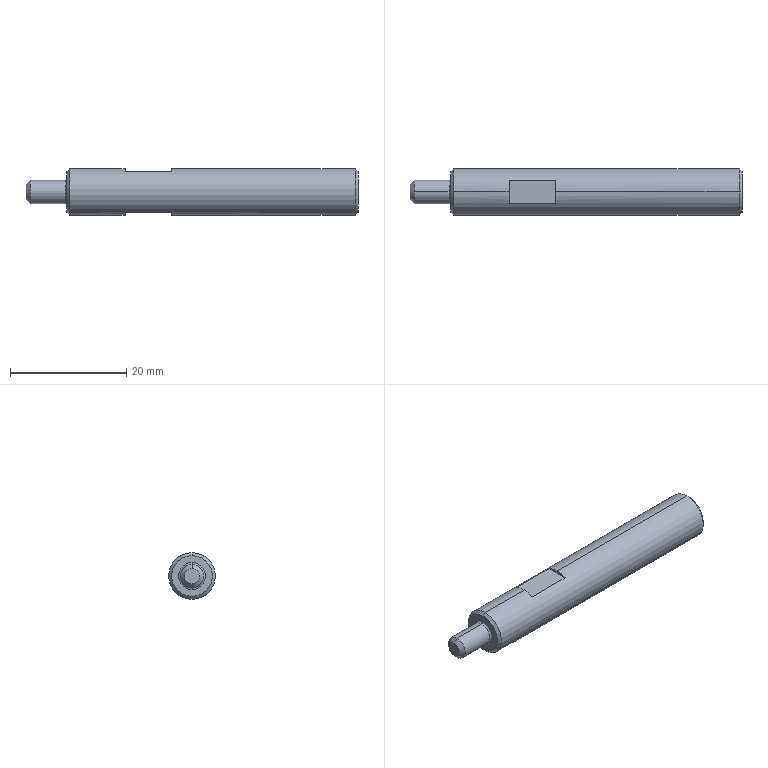Part | STEP file | PSSGGZ8-50-F7-B5-P4-N5-SC10 | 1 solid | 27 faces | box 57 x 8 x 8 mm | volume 2360 mm3 | cone 10 | plane 9 | cylinder 6 | torus 2 | commonest cylinder face diameters 4 x2 4.134 x2 8 x2
STEP:
#1=CARTESIAN_POINT('',(49.567,0.,2.067));
#2=VERTEX_POINT('',#1);
#3=CARTESIAN_POINT('',(49.567,0.,-2.067));
#4=VERTEX_POINT('',#3);
#5=CARTESIAN_POINT('',(49.567,0.,0.));
#6=DIRECTION('',(1.,0.,0.));
#7=DIRECTION('',(0.,0.,-1.));
#8=AXIS2_PLACEMENT_3D('',#5,#6,#7);
#9=CIRCLE('',#8,2.067);
#10=EDGE_CURVE('',#2,#4,#9,.T.);
#11=ORIENTED_EDGE('',*,*,#10,.F.);
#12=CARTESIAN_POINT('',(50.,0.,2.5));
#13=VERTEX_POINT('',#12);
#14=CARTESIAN_POINT('',(49.567,0.,2.067));
#15=DIRECTION('',(0.7071,0.,0.7071));
#16=VECTOR('',#15,1000.);
#17=LINE('',#14,#16);
#18=EDGE_CURVE('',#2,#13,#17,.T.);
#19=ORIENTED_EDGE('',*,*,#18,.T.);
#20=CARTESIAN_POINT('',(50.,0.,-2.5));
#21=VERTEX_POINT('',#20);
#22=CARTESIAN_POINT('',(50.,0.,0.));
#23=DIRECTION('',(1.,0.,0.));
#24=DIRECTION('',(0.,0.,-1.));
#25=AXIS2_PLACEMENT_3D('',#22,#23,#24);
#26=CIRCLE('',#25,2.5);
#27=EDGE_CURVE('',#13,#21,#26,.T.);
#28=ORIENTED_EDGE('',*,*,#27,.T.);
#29=CARTESIAN_POINT('',(49.567,0.,-2.067));
#30=DIRECTION('',(0.7071,0.,-0.7071));
#31=VECTOR('',#30,1000.);
#32=LINE('',#29,#31);
#33=EDGE_CURVE('',#4,#21,#32,.T.);
#34=ORIENTED_EDGE('',*,*,#33,.F.);
#35=EDGE_LOOP('',(#11,#19,#28,#34));
#36=FACE_OUTER_BOUND('',#35,.T.);
#37=CARTESIAN_POINT('',(49.567,0.,0.));
#38=DIRECTION('',(1.,0.,0.));
#39=DIRECTION('',(0.,0.,-1.));
#40=AXIS2_PLACEMENT_3D('',#37,#38,#39);
#41=CONICAL_SURFACE('',#40,2.067,0.7854);
#42=ADVANCED_FACE('',(#36),#41,.F.);
#43=CARTESIAN_POINT('',(50.,0.,-3.5));
#44=VERTEX_POINT('',#43);
#45=CARTESIAN_POINT('',(50.,0.,3.5));
#46=VERTEX_POINT('',#45);
#47=CARTESIAN_POINT('',(50.,0.,0.));
#48=DIRECTION('',(1.,0.,0.));
#49=DIRECTION('',(0.,0.,-1.));
#50=AXIS2_PLACEMENT_3D('',#47,#48,#49);
#51=CIRCLE('',#50,3.5);
#52=EDGE_CURVE('',#44,#46,#51,.T.);
#53=ORIENTED_EDGE('',*,*,#52,.F.);
#54=CARTESIAN_POINT('',(49.5,0.,-4.));
#55=VERTEX_POINT('',#54);
#56=CARTESIAN_POINT('',(49.5,0.,-4.));
#57=DIRECTION('',(-0.7071,0.,-0.7071));
#58=VECTOR('',#57,1000.);
#59=LINE('',#56,#58);
#60=EDGE_CURVE('',#44,#55,#59,.T.);
#61=ORIENTED_EDGE('',*,*,#60,.T.);
#62=CARTESIAN_POINT('',(49.5,0.,4.));
#63=VERTEX_POINT('',#62);
#64=CARTESIAN_POINT('',(49.5,0.,0.));
#65=DIRECTION('',(1.,0.,0.));
#66=DIRECTION('',(0.,0.,-1.));
#67=AXIS2_PLACEMENT_3D('',#64,#65,#66);
#68=CIRCLE('',#67,4.);
#69=EDGE_CURVE('',#55,#63,#68,.T.);
#70=ORIENTED_EDGE('',*,*,#69,.T.);
#71=CARTESIAN_POINT('',(49.5,0.,4.));
#72=DIRECTION('',(-0.7071,0.,0.7071));
#73=VECTOR('',#72,1000.);
#74=LINE('',#71,#73);
#75=EDGE_CURVE('',#46,#63,#74,.T.);
#76=ORIENTED_EDGE('',*,*,#75,.F.);
#77=EDGE_LOOP('',(#53,#61,#70,#76));
#78=FACE_OUTER_BOUND('',#77,.T.);
#79=CARTESIAN_POINT('',(49.5,0.,0.));
#80=DIRECTION('',(-1.,0.,0.));
#81=DIRECTION('',(0.,0.,1.));
#82=AXIS2_PLACEMENT_3D('',#79,#80,#81);
#83=CONICAL_SURFACE('',#82,4.,0.7854);
#84=ADVANCED_FACE('',(#78),#83,.T.);
#85=CARTESIAN_POINT('',(49.5,0.,0.));
#86=DIRECTION('',(1.,0.,0.));
#87=DIRECTION('',(0.,0.,-1.));
#88=AXIS2_PLACEMENT_3D('',#85,#86,#87);
#89=CIRCLE('',#88,4.);
#90=EDGE_CURVE('',#63,#55,#89,.T.);
#91=ORIENTED_EDGE('',*,*,#90,.F.);
#92=CARTESIAN_POINT('',(18.,0.,4.));
#93=VERTEX_POINT('',#92);
#94=CARTESIAN_POINT('',(50.,0.,4.));
#95=DIRECTION('',(-1.,0.,0.));
#96=VECTOR('',#95,1000.);
#97=LINE('',#94,#96);
#98=EDGE_CURVE('',#63,#93,#97,.T.);
#99=ORIENTED_EDGE('',*,*,#98,.T.);
#100=CARTESIAN_POINT('',(18.,-1.936,3.5));
#101=VERTEX_POINT('',#100);
#102=CARTESIAN_POINT('',(18.,0.,0.));
#103=DIRECTION('',(1.,0.,0.));
#104=DIRECTION('',(0.,0.,-1.));
#105=AXIS2_PLACEMENT_3D('',#102,#103,#104);
#106=CIRCLE('',#105,4.);
#107=EDGE_CURVE('',#93,#101,#106,.T.);
#108=ORIENTED_EDGE('',*,*,#107,.T.);
#109=CARTESIAN_POINT('',(10.,-1.936,3.5));
#110=VERTEX_POINT('',#109);
#111=CARTESIAN_POINT('',(50.,-1.936,3.5));
#112=DIRECTION('',(-1.,0.,0.));
#113=VECTOR('',#112,1000.);
#114=LINE('',#111,#113);
#115=EDGE_CURVE('',#101,#110,#114,.T.);
#116=ORIENTED_EDGE('',*,*,#115,.T.);
#117=CARTESIAN_POINT('',(10.,0.,4.));
#118=VERTEX_POINT('',#117);
#119=CARTESIAN_POINT('',(10.,0.,0.));
#120=DIRECTION('',(1.,0.,0.));
#121=DIRECTION('',(0.,0.,-1.));
#122=AXIS2_PLACEMENT_3D('',#119,#120,#121);
#123=CIRCLE('',#122,4.);
#124=EDGE_CURVE('',#118,#110,#123,.T.);
#125=ORIENTED_EDGE('',*,*,#124,.F.);
#126=CARTESIAN_POINT('',(0.5,0.,4.));
#127=VERTEX_POINT('',#126);
#128=CARTESIAN_POINT('',(50.,0.,4.));
#129=DIRECTION('',(-1.,0.,0.));
#130=VECTOR('',#129,1000.);
#131=LINE('',#128,#130);
#132=EDGE_CURVE('',#118,#127,#131,.T.);
#133=ORIENTED_EDGE('',*,*,#132,.T.);
#134=CARTESIAN_POINT('',(0.5,0.,-4.));
#135=VERTEX_POINT('',#134);
#136=CARTESIAN_POINT('',(0.5,0.,0.));
#137=DIRECTION('',(1.,0.,0.));
#138=DIRECTION('',(0.,0.,-1.));
#139=AXIS2_PLACEMENT_3D('',#136,#137,#138);
#140=CIRCLE('',#139,4.);
#141=EDGE_CURVE('',#127,#135,#140,.T.);
#142=ORIENTED_EDGE('',*,*,#141,.T.);
#143=CARTESIAN_POINT('',(10.,0.,-4.));
#144=VERTEX_POINT('',#143);
#145=CARTESIAN_POINT('',(50.,0.,-4.));
#146=DIRECTION('',(-1.,0.,0.));
#147=VECTOR('',#146,1000.);
#148=LINE('',#145,#147);
#149=EDGE_CURVE('',#144,#135,#148,.T.);
#150=ORIENTED_EDGE('',*,*,#149,.F.);
#151=CARTESIAN_POINT('',(10.,-1.936,-3.5));
#152=VERTEX_POINT('',#151);
#153=CARTESIAN_POINT('',(10.,0.,0.));
#154=DIRECTION('',(1.,0.,0.));
#155=DIRECTION('',(0.,0.,-1.));
#156=AXIS2_PLACEMENT_3D('',#153,#154,#155);
#157=CIRCLE('',#156,4.);
#158=EDGE_CURVE('',#152,#144,#157,.T.);
#159=ORIENTED_EDGE('',*,*,#158,.F.);
#160=CARTESIAN_POINT('',(18.,-1.936,-3.5));
#161=VERTEX_POINT('',#160);
#162=CARTESIAN_POINT('',(50.,-1.936,-3.5));
#163=DIRECTION('',(1.,0.,0.));
#164=VECTOR('',#163,1000.);
#165=LINE('',#162,#164);
#166=EDGE_CURVE('',#152,#161,#165,.T.);
#167=ORIENTED_EDGE('',*,*,#166,.T.);
#168=CARTESIAN_POINT('',(18.,0.,-4.));
#169=VERTEX_POINT('',#168);
#170=CARTESIAN_POINT('',(18.,0.,0.));
#171=DIRECTION('',(1.,0.,0.));
#172=DIRECTION('',(0.,0.,-1.));
#173=AXIS2_PLACEMENT_3D('',#170,#171,#172);
#174=CIRCLE('',#173,4.);
#175=EDGE_CURVE('',#161,#169,#174,.T.);
#176=ORIENTED_EDGE('',*,*,#175,.T.);
#177=CARTESIAN_POINT('',(50.,0.,-4.));
#178=DIRECTION('',(-1.,0.,0.));
#179=VECTOR('',#178,1000.);
#180=LINE('',#177,#179);
#181=EDGE_CURVE('',#55,#169,#180,.T.);
#182=ORIENTED_EDGE('',*,*,#181,.F.);
#183=EDGE_LOOP('',(#91,#99,#108,#116,#125,#133,#142,#150,#159,#167,#176,#182));
#184=FACE_OUTER_BOUND('',#183,.T.);
#185=CARTESIAN_POINT('',(50.,0.,0.));
#186=DIRECTION('',(-1.,0.,0.));
#187=DIRECTION('',(0.,0.,-1.));
#188=AXIS2_PLACEMENT_3D('',#185,#186,#187);
#189=CYLINDRICAL_SURFACE('',#188,4.);
#190=ADVANCED_FACE('',(#184),#189,.T.);
#191=CARTESIAN_POINT('',(0.,0.,-3.5));
#192=VERTEX_POINT('',#191);
#193=CARTESIAN_POINT('',(0.,0.,3.5));
#194=VERTEX_POINT('',#193);
#195=CARTESIAN_POINT('',(0.,0.,0.));
#196=DIRECTION('',(1.,0.,0.));
#197=DIRECTION('',(0.,0.,-1.));
#198=AXIS2_PLACEMENT_3D('',#195,#196,#197);
#199=CIRCLE('',#198,3.5);
#200=EDGE_CURVE('',#192,#194,#199,.T.);
#201=ORIENTED_EDGE('',*,*,#200,.T.);
#202=CARTESIAN_POINT('',(0.,0.,3.5));
#203=DIRECTION('',(0.7071,0.,0.7071));
#204=VECTOR('',#203,1000.);
#205=LINE('',#202,#204);
#206=EDGE_CURVE('',#194,#127,#205,.T.);
#207=ORIENTED_EDGE('',*,*,#206,.T.);
#208=CARTESIAN_POINT('',(0.5,0.,0.));
#209=DIRECTION('',(1.,0.,0.));
#210=DIRECTION('',(0.,0.,-1.));
#211=AXIS2_PLACEMENT_3D('',#208,#209,#210);
#212=CIRCLE('',#211,4.);
#213=EDGE_CURVE('',#135,#127,#212,.T.);
#214=ORIENTED_EDGE('',*,*,#213,.F.);
#215=CARTESIAN_POINT('',(0.,0.,-3.5));
#216=DIRECTION('',(0.7071,0.,-0.7071));
#217=VECTOR('',#216,1000.);
#218=LINE('',#215,#217);
#219=EDGE_CURVE('',#192,#135,#218,.T.);
#220=ORIENTED_EDGE('',*,*,#219,.F.);
#221=EDGE_LOOP('',(#201,#207,#214,#220));
#222=FACE_OUTER_BOUND('',#221,.T.);
#223=CARTESIAN_POINT('',(0.,0.,0.));
#224=DIRECTION('',(1.,0.,0.));
#225=DIRECTION('',(0.,0.,-1.));
#226=AXIS2_PLACEMENT_3D('',#223,#224,#225);
#227=CONICAL_SURFACE('',#226,3.5,0.7854);
#228=ADVANCED_FACE('',(#222),#227,.T.);
#229=CARTESIAN_POINT('',(0.,0.,2.3));
#230=VERTEX_POINT('',#229);
#231=CARTESIAN_POINT('',(0.,0.,-2.3));
#232=VERTEX_POINT('',#231);
#233=CARTESIAN_POINT('',(0.,0.,0.));
#234=DIRECTION('',(1.,0.,0.));
#235=DIRECTION('',(0.,0.,-1.));
#236=AXIS2_PLACEMENT_3D('',#233,#234,#235);
#237=CIRCLE('',#236,2.3);
#238=EDGE_CURVE('',#230,#232,#237,.T.);
#239=ORIENTED_EDGE('',*,*,#238,.F.);
#240=CARTESIAN_POINT('',(-0.3,0.,2.));
#241=VERTEX_POINT('',#240);
#242=CARTESIAN_POINT('',(-0.3,0.,2.3));
#243=DIRECTION('',(0.,1.,0.));
#244=DIRECTION('',(0.,0.,1.));
#245=AXIS2_PLACEMENT_3D('',#242,#243,#244);
#246=CIRCLE('',#245,0.3);
#247=EDGE_CURVE('',#230,#241,#246,.T.);
#248=ORIENTED_EDGE('',*,*,#247,.T.);
#249=CARTESIAN_POINT('',(-0.3,0.,-2.));
#250=VERTEX_POINT('',#249);
#251=CARTESIAN_POINT('',(-0.3,0.,0.));
#252=DIRECTION('',(1.,0.,0.));
#253=DIRECTION('',(0.,0.,-1.));
#254=AXIS2_PLACEMENT_3D('',#251,#252,#253);
#255=CIRCLE('',#254,2.);
#256=EDGE_CURVE('',#241,#250,#255,.T.);
#257=ORIENTED_EDGE('',*,*,#256,.T.);
#258=CARTESIAN_POINT('',(-0.3,0.,-2.3));
#259=DIRECTION('',(0.,-1.,0.));
#260=DIRECTION('',(0.,0.,-1.));
#261=AXIS2_PLACEMENT_3D('',#258,#259,#260);
#262=CIRCLE('',#261,0.3);
#263=EDGE_CURVE('',#232,#250,#262,.T.);
#264=ORIENTED_EDGE('',*,*,#263,.F.);
#265=EDGE_LOOP('',(#239,#248,#257,#264));
#266=FACE_OUTER_BOUND('',#265,.T.);
#267=CARTESIAN_POINT('',(-0.3,0.,0.));
#268=DIRECTION('',(1.,0.,0.));
#269=DIRECTION('',(0.,0.,-1.));
#270=AXIS2_PLACEMENT_3D('',#267,#268,#269);
#271=TOROIDAL_SURFACE('',#270,2.3,0.3);
#272=ADVANCED_FACE('',(#266),#271,.F.);
#273=ORIENTED_EDGE('',*,*,#256,.F.);
#274=CARTESIAN_POINT('',(-6.3,0.,2.));
#275=VERTEX_POINT('',#274);
#276=CARTESIAN_POINT('',(50.,0.,2.));
#277=DIRECTION('',(-1.,0.,0.));
#278=VECTOR('',#277,1000.);
#279=LINE('',#276,#278);
#280=EDGE_CURVE('',#241,#275,#279,.T.);
#281=ORIENTED_EDGE('',*,*,#280,.T.);
#282=CARTESIAN_POINT('',(-6.3,0.,-2.));
#283=VERTEX_POINT('',#282);
#284=CARTESIAN_POINT('',(-6.3,0.,0.));
#285=DIRECTION('',(1.,0.,0.));
#286=DIRECTION('',(0.,0.,-1.));
#287=AXIS2_PLACEMENT_3D('',#284,#285,#286);
#288=CIRCLE('',#287,2.);
#289=EDGE_CURVE('',#275,#283,#288,.T.);
#290=ORIENTED_EDGE('',*,*,#289,.T.);
#291=CARTESIAN_POINT('',(50.,0.,-2.));
#292=DIRECTION('',(-1.,0.,0.));
#293=VECTOR('',#292,1000.);
#294=LINE('',#291,#293);
#295=EDGE_CURVE('',#250,#283,#294,.T.);
#296=ORIENTED_EDGE('',*,*,#295,.F.);
#297=EDGE_LOOP('',(#273,#281,#290,#296));
#298=FACE_OUTER_BOUND('',#297,.T.);
#299=CARTESIAN_POINT('',(50.,0.,0.));
#300=DIRECTION('',(-1.,0.,0.));
#301=DIRECTION('',(0.,0.,-1.));
#302=AXIS2_PLACEMENT_3D('',#299,#300,#301);
#303=CYLINDRICAL_SURFACE('',#302,2.);
#304=ADVANCED_FACE('',(#298),#303,.T.);
#305=CARTESIAN_POINT('',(-7.,0.,-1.3));
#306=VERTEX_POINT('',#305);
#307=CARTESIAN_POINT('',(-7.,0.,1.3));
#308=VERTEX_POINT('',#307);
#309=CARTESIAN_POINT('',(-7.,0.,0.));
#310=DIRECTION('',(1.,0.,0.));
#311=DIRECTION('',(0.,0.,-1.));
#312=AXIS2_PLACEMENT_3D('',#309,#310,#311);
#313=CIRCLE('',#312,1.3);
#314=EDGE_CURVE('',#306,#308,#313,.T.);
#315=ORIENTED_EDGE('',*,*,#314,.T.);
#316=CARTESIAN_POINT('',(-7.,0.,1.3));
#317=DIRECTION('',(0.7071,0.,0.7071));
#318=VECTOR('',#317,1000.);
#319=LINE('',#316,#318);
#320=EDGE_CURVE('',#308,#275,#319,.T.);
#321=ORIENTED_EDGE('',*,*,#320,.T.);
#322=CARTESIAN_POINT('',(-6.3,0.,0.));
#323=DIRECTION('',(1.,0.,0.));
#324=DIRECTION('',(0.,0.,-1.));
#325=AXIS2_PLACEMENT_3D('',#322,#323,#324);
#326=CIRCLE('',#325,2.);
#327=EDGE_CURVE('',#283,#275,#326,.T.);
#328=ORIENTED_EDGE('',*,*,#327,.F.);
#329=CARTESIAN_POINT('',(-7.,0.,-1.3));
#330=DIRECTION('',(0.7071,0.,-0.7071));
#331=VECTOR('',#330,1000.);
#332=LINE('',#329,#331);
#333=EDGE_CURVE('',#306,#283,#332,.T.);
#334=ORIENTED_EDGE('',*,*,#333,.F.);
#335=EDGE_LOOP('',(#315,#321,#328,#334));
#336=FACE_OUTER_BOUND('',#335,.T.);
#337=CARTESIAN_POINT('',(-7.,0.,0.));
#338=DIRECTION('',(1.,0.,0.));
#339=DIRECTION('',(0.,0.,-1.));
#340=AXIS2_PLACEMENT_3D('',#337,#338,#339);
#341=CONICAL_SURFACE('',#340,1.3,0.7854);
#342=ADVANCED_FACE('',(#336),#341,.T.);
#343=CARTESIAN_POINT('',(49.567,0.,0.));
#344=DIRECTION('',(1.,0.,0.));
#345=DIRECTION('',(0.,0.,-1.));
#346=AXIS2_PLACEMENT_3D('',#343,#344,#345);
#347=CIRCLE('',#346,2.067);
#348=EDGE_CURVE('',#4,#2,#347,.T.);
#349=ORIENTED_EDGE('',*,*,#348,.T.);
#350=CARTESIAN_POINT('',(34.693,0.,2.067));
#351=VERTEX_POINT('',#350);
#352=CARTESIAN_POINT('',(50.,0.,2.067));
#353=DIRECTION('',(-1.,0.,0.));
#354=VECTOR('',#353,1000.);
#355=LINE('',#352,#354);
#356=EDGE_CURVE('',#2,#351,#355,.T.);
#357=ORIENTED_EDGE('',*,*,#356,.T.);
#358=CARTESIAN_POINT('',(34.693,0.,-2.067));
#359=VERTEX_POINT('',#358);
#360=CARTESIAN_POINT('',(34.693,0.,0.));
#361=DIRECTION('',(1.,0.,0.));
#362=DIRECTION('',(0.,0.,-1.));
#363=AXIS2_PLACEMENT_3D('',#360,#361,#362);
#364=CIRCLE('',#363,2.067);
#365=EDGE_CURVE('',#359,#351,#364,.T.);
#366=ORIENTED_EDGE('',*,*,#365,.F.);
#367=CARTESIAN_POINT('',(50.,0.,-2.067));
#368=DIRECTION('',(-1.,0.,0.));
#369=VECTOR('',#368,1000.);
#370=LINE('',#367,#369);
#371=EDGE_CURVE('',#4,#359,#370,.T.);
#372=ORIENTED_EDGE('',*,*,#371,.F.);
#373=EDGE_LOOP('',(#349,#357,#366,#372));
#374=FACE_OUTER_BOUND('',#373,.T.);
#375=CARTESIAN_POINT('',(50.,0.,0.));
#376=DIRECTION('',(-1.,0.,0.));
#377=DIRECTION('',(0.,0.,-1.));
#378=AXIS2_PLACEMENT_3D('',#375,#376,#377);
#379=CYLINDRICAL_SURFACE('',#378,2.067);
#380=ADVANCED_FACE('',(#374),#379,.F.);
#381=CARTESIAN_POINT('',(33.5,0.,0.));
#382=VERTEX_POINT('',#381);
#383=CARTESIAN_POINT('',(533.5,0.,-866.025));
#384=DIRECTION('',(0.5,0.,-0.866));
#385=VECTOR('',#384,1000.);
#386=LINE('',#383,#385);
#387=EDGE_CURVE('',#382,#359,#386,.T.);
#388=ORIENTED_EDGE('',*,*,#387,.F.);
#389=CARTESIAN_POINT('',(533.5,0.,866.025));
#390=DIRECTION('',(0.5,0.,0.866));
#391=VECTOR('',#390,1000.);
#392=LINE('',#389,#391);
#393=EDGE_CURVE('',#382,#351,#392,.T.);
#394=ORIENTED_EDGE('',*,*,#393,.T.);
#395=CARTESIAN_POINT('',(34.693,0.,0.));
#396=DIRECTION('',(1.,0.,0.));
#397=DIRECTION('',(0.,0.,-1.));
#398=AXIS2_PLACEMENT_3D('',#395,#396,#397);
#399=CIRCLE('',#398,2.067);
#400=EDGE_CURVE('',#351,#359,#399,.T.);
#401=ORIENTED_EDGE('',*,*,#400,.T.);
#402=EDGE_LOOP('',(#388,#394,#401));
#403=FACE_OUTER_BOUND('',#402,.T.);
#404=CARTESIAN_POINT('',(533.5,0.,0.));
#405=DIRECTION('',(1.,0.,0.));
#406=DIRECTION('',(0.,0.,-1.));
#407=AXIS2_PLACEMENT_3D('',#404,#405,#406);
#408=CONICAL_SURFACE('',#407,866.025,1.047);
#409=ADVANCED_FACE('',(#403),#408,.F.);
#410=ORIENTED_EDGE('',*,*,#393,.F.);
#411=ORIENTED_EDGE('',*,*,#387,.T.);
#412=ORIENTED_EDGE('',*,*,#365,.T.);
#413=EDGE_LOOP('',(#410,#411,#412));
#414=FACE_OUTER_BOUND('',#413,.T.);
#415=CARTESIAN_POINT('',(533.5,0.,0.));
#416=DIRECTION('',(1.,0.,0.));
#417=DIRECTION('',(0.,0.,-1.));
#418=AXIS2_PLACEMENT_3D('',#415,#416,#417);
#419=CONICAL_SURFACE('',#418,866.025,1.047);
#420=ADVANCED_FACE('',(#414),#419,.F.);
#421=ORIENTED_EDGE('',*,*,#356,.F.);
#422=ORIENTED_EDGE('',*,*,#10,.T.);
#423=ORIENTED_EDGE('',*,*,#371,.T.);
#424=ORIENTED_EDGE('',*,*,#400,.F.);
#425=EDGE_LOOP('',(#421,#422,#423,#424));
#426=FACE_OUTER_BOUND('',#425,.T.);
#427=CARTESIAN_POINT('',(50.,0.,0.));
#428=DIRECTION('',(-1.,0.,0.));
#429=DIRECTION('',(0.,0.,-1.));
#430=AXIS2_PLACEMENT_3D('',#427,#428,#429);
#431=CYLINDRICAL_SURFACE('',#430,2.067);
#432=ADVANCED_FACE('',(#426),#431,.F.);
#433=CARTESIAN_POINT('',(10.,1.936,3.5));
#434=VERTEX_POINT('',#433);
#435=CARTESIAN_POINT('',(10.,0.,0.));
#436=DIRECTION('',(1.,0.,0.));
#437=DIRECTION('',(0.,0.,-1.));
#438=AXIS2_PLACEMENT_3D('',#435,#436,#437);
#439=CIRCLE('',#438,4.);
#440=EDGE_CURVE('',#434,#118,#439,.T.);
#441=ORIENTED_EDGE('',*,*,#440,.T.);
#442=ORIENTED_EDGE('',*,*,#124,.T.);
#443=CARTESIAN_POINT('',(10.,8.,3.5));
#444=DIRECTION('',(0.,-1.,0.));
#445=VECTOR('',#444,1000.);
#446=LINE('',#443,#445);
#447=EDGE_CURVE('',#434,#110,#446,.T.);
#448=ORIENTED_EDGE('',*,*,#447,.F.);
#449=EDGE_LOOP('',(#441,#442,#448));
#450=FACE_OUTER_BOUND('',#449,.T.);
#451=CARTESIAN_POINT('',(10.,0.,0.));
#452=DIRECTION('',(1.,0.,0.));
#453=DIRECTION('',(0.,0.,-1.));
#454=AXIS2_PLACEMENT_3D('',#451,#452,#453);
#455=PLANE('',#454);
#456=ADVANCED_FACE('',(#450),#455,.T.);
#457=ORIENTED_EDGE('',*,*,#314,.F.);
#458=CARTESIAN_POINT('',(-7.,0.,0.));
#459=DIRECTION('',(1.,0.,0.));
#460=DIRECTION('',(0.,0.,-1.));
#461=AXIS2_PLACEMENT_3D('',#458,#459,#460);
#462=CIRCLE('',#461,1.3);
#463=EDGE_CURVE('',#308,#306,#462,.T.);
#464=ORIENTED_EDGE('',*,*,#463,.F.);
#465=EDGE_LOOP('',(#457,#464));
#466=FACE_OUTER_BOUND('',#465,.T.);
#467=CARTESIAN_POINT('',(-7.,0.,0.));
#468=DIRECTION('',(1.,0.,0.));
#469=DIRECTION('',(0.,0.,-1.));
#470=AXIS2_PLACEMENT_3D('',#467,#468,#469);
#471=PLANE('',#470);
#472=ADVANCED_FACE('',(#466),#471,.F.);
#473=ORIENTED_EDGE('',*,*,#320,.F.);
#474=ORIENTED_EDGE('',*,*,#463,.T.);
#475=ORIENTED_EDGE('',*,*,#333,.T.);
#476=ORIENTED_EDGE('',*,*,#289,.F.);
#477=EDGE_LOOP('',(#473,#474,#475,#476));
#478=FACE_OUTER_BOUND('',#477,.T.);
#479=CARTESIAN_POINT('',(-7.,0.,0.));
#480=DIRECTION('',(1.,0.,0.));
#481=DIRECTION('',(0.,0.,-1.));
#482=AXIS2_PLACEMENT_3D('',#479,#480,#481);
#483=CONICAL_SURFACE('',#482,1.3,0.7854);
#484=ADVANCED_FACE('',(#478),#483,.T.);
#485=ORIENTED_EDGE('',*,*,#280,.F.);
#486=CARTESIAN_POINT('',(-0.3,0.,0.));
#487=DIRECTION('',(1.,0.,0.));
#488=DIRECTION('',(0.,0.,-1.));
#489=AXIS2_PLACEMENT_3D('',#486,#487,#488);
#490=CIRCLE('',#489,2.);
#491=EDGE_CURVE('',#250,#241,#490,.T.);
#492=ORIENTED_EDGE('',*,*,#491,.F.);
#493=ORIENTED_EDGE('',*,*,#295,.T.);
#494=ORIENTED_EDGE('',*,*,#327,.T.);
#495=EDGE_LOOP('',(#485,#492,#493,#494));
#496=FACE_OUTER_BOUND('',#495,.T.);
#497=CARTESIAN_POINT('',(50.,0.,0.));
#498=DIRECTION('',(-1.,0.,0.));
#499=DIRECTION('',(0.,0.,-1.));
#500=AXIS2_PLACEMENT_3D('',#497,#498,#499);
#501=CYLINDRICAL_SURFACE('',#500,2.);
#502=ADVANCED_FACE('',(#496),#501,.T.);
#503=ORIENTED_EDGE('',*,*,#247,.F.);
#504=CARTESIAN_POINT('',(0.,0.,0.));
#505=DIRECTION('',(1.,0.,0.));
#506=DIRECTION('',(0.,0.,-1.));
#507=AXIS2_PLACEMENT_3D('',#504,#505,#506);
#508=CIRCLE('',#507,2.3);
#509=EDGE_CURVE('',#232,#230,#508,.T.);
#510=ORIENTED_EDGE('',*,*,#509,.F.);
#511=ORIENTED_EDGE('',*,*,#263,.T.);
#512=ORIENTED_EDGE('',*,*,#491,.T.);
#513=EDGE_LOOP('',(#503,#510,#511,#512));
#514=FACE_OUTER_BOUND('',#513,.T.);
#515=CARTESIAN_POINT('',(-0.3,0.,0.));
#516=DIRECTION('',(1.,0.,0.));
#517=DIRECTION('',(0.,0.,-1.));
#518=AXIS2_PLACEMENT_3D('',#515,#516,#517);
#519=TOROIDAL_SURFACE('',#518,2.3,0.3);
#520=ADVANCED_FACE('',(#514),#519,.F.);
#521=ORIENTED_EDGE('',*,*,#200,.F.);
#522=CARTESIAN_POINT('',(0.,0.,0.));
#523=DIRECTION('',(1.,0.,0.));
#524=DIRECTION('',(0.,0.,-1.));
#525=AXIS2_PLACEMENT_3D('',#522,#523,#524);
#526=CIRCLE('',#525,3.5);
#527=EDGE_CURVE('',#194,#192,#526,.T.);
#528=ORIENTED_EDGE('',*,*,#527,.F.);
#529=EDGE_LOOP('',(#521,#528));
#530=FACE_OUTER_BOUND('',#529,.T.);
#531=ORIENTED_EDGE('',*,*,#509,.T.);
#532=ORIENTED_EDGE('',*,*,#238,.T.);
#533=EDGE_LOOP('',(#531,#532));
#534=FACE_BOUND('',#533,.T.);
#535=CARTESIAN_POINT('',(0.,2.3,0.));
#536=DIRECTION('',(1.,0.,0.));
#537=DIRECTION('',(0.,0.,-1.));
#538=AXIS2_PLACEMENT_3D('',#535,#536,#537);
#539=PLANE('',#538);
#540=ADVANCED_FACE('',(#530,#534),#539,.F.);
#541=ORIENTED_EDGE('',*,*,#206,.F.);
#542=ORIENTED_EDGE('',*,*,#527,.T.);
#543=ORIENTED_EDGE('',*,*,#219,.T.);
#544=ORIENTED_EDGE('',*,*,#141,.F.);
#545=EDGE_LOOP('',(#541,#542,#543,#544));
#546=FACE_OUTER_BOUND('',#545,.T.);
#547=CARTESIAN_POINT('',(0.,0.,0.));
#548=DIRECTION('',(1.,0.,0.));
#549=DIRECTION('',(0.,0.,-1.));
#550=AXIS2_PLACEMENT_3D('',#547,#548,#549);
#551=CONICAL_SURFACE('',#550,3.5,0.7854);
#552=ADVANCED_FACE('',(#546),#551,.T.);
#553=ORIENTED_EDGE('',*,*,#98,.F.);
#554=ORIENTED_EDGE('',*,*,#69,.F.);
#555=ORIENTED_EDGE('',*,*,#181,.T.);
#556=CARTESIAN_POINT('',(18.,1.936,-3.5));
#557=VERTEX_POINT('',#556);
#558=CARTESIAN_POINT('',(18.,0.,0.));
#559=DIRECTION('',(1.,0.,0.));
#560=DIRECTION('',(0.,0.,-1.));
#561=AXIS2_PLACEMENT_3D('',#558,#559,#560);
#562=CIRCLE('',#561,4.);
#563=EDGE_CURVE('',#169,#557,#562,.T.);
#564=ORIENTED_EDGE('',*,*,#563,.T.);
#565=CARTESIAN_POINT('',(10.,1.936,-3.5));
#566=VERTEX_POINT('',#565);
#567=CARTESIAN_POINT('',(50.,1.936,-3.5));
#568=DIRECTION('',(-1.,0.,0.));
#569=VECTOR('',#568,1000.);
#570=LINE('',#567,#569);
#571=EDGE_CURVE('',#557,#566,#570,.T.);
#572=ORIENTED_EDGE('',*,*,#571,.T.);
#573=CARTESIAN_POINT('',(10.,0.,0.));
#574=DIRECTION('',(1.,0.,0.));
#575=DIRECTION('',(0.,0.,-1.));
#576=AXIS2_PLACEMENT_3D('',#573,#574,#575);
#577=CIRCLE('',#576,4.);
#578=EDGE_CURVE('',#144,#566,#577,.T.);
#579=ORIENTED_EDGE('',*,*,#578,.F.);
#580=ORIENTED_EDGE('',*,*,#149,.T.);
#581=ORIENTED_EDGE('',*,*,#213,.T.);
#582=ORIENTED_EDGE('',*,*,#132,.F.);
#583=ORIENTED_EDGE('',*,*,#440,.F.);
#584=CARTESIAN_POINT('',(18.,1.936,3.5));
#585=VERTEX_POINT('',#584);
#586=CARTESIAN_POINT('',(50.,1.936,3.5));
#587=DIRECTION('',(1.,0.,0.));
#588=VECTOR('',#587,1000.);
#589=LINE('',#586,#588);
#590=EDGE_CURVE('',#434,#585,#589,.T.);
#591=ORIENTED_EDGE('',*,*,#590,.T.);
#592=CARTESIAN_POINT('',(18.,0.,0.));
#593=DIRECTION('',(1.,0.,0.));
#594=DIRECTION('',(0.,0.,-1.));
#595=AXIS2_PLACEMENT_3D('',#592,#593,#594);
#596=CIRCLE('',#595,4.);
#597=EDGE_CURVE('',#585,#93,#596,.T.);
#598=ORIENTED_EDGE('',*,*,#597,.T.);
#599=EDGE_LOOP('',(#553,#554,#555,#564,#572,#579,#580,#581,#582,#583,#591,#598));
#600=FACE_OUTER_BOUND('',#599,.T.);
#601=CARTESIAN_POINT('',(50.,0.,0.));
#602=DIRECTION('',(-1.,0.,0.));
#603=DIRECTION('',(0.,0.,-1.));
#604=AXIS2_PLACEMENT_3D('',#601,#602,#603);
#605=CYLINDRICAL_SURFACE('',#604,4.);
#606=ADVANCED_FACE('',(#600),#605,.T.);
#607=ORIENTED_EDGE('',*,*,#60,.F.);
#608=CARTESIAN_POINT('',(50.,0.,0.));
#609=DIRECTION('',(1.,0.,0.));
#610=DIRECTION('',(0.,0.,-1.));
#611=AXIS2_PLACEMENT_3D('',#608,#609,#610);
#612=CIRCLE('',#611,3.5);
#613=EDGE_CURVE('',#46,#44,#612,.T.);
#614=ORIENTED_EDGE('',*,*,#613,.F.);
#615=ORIENTED_EDGE('',*,*,#75,.T.);
#616=ORIENTED_EDGE('',*,*,#90,.T.);
#617=EDGE_LOOP('',(#607,#614,#615,#616));
#618=FACE_OUTER_BOUND('',#617,.T.);
#619=CARTESIAN_POINT('',(49.5,0.,0.));
#620=DIRECTION('',(-1.,0.,0.));
#621=DIRECTION('',(0.,0.,1.));
#622=AXIS2_PLACEMENT_3D('',#619,#620,#621);
#623=CONICAL_SURFACE('',#622,4.,0.7854);
#624=ADVANCED_FACE('',(#618),#623,.T.);
#625=CARTESIAN_POINT('',(50.,0.,0.));
#626=DIRECTION('',(1.,0.,0.));
#627=DIRECTION('',(0.,0.,-1.));
#628=AXIS2_PLACEMENT_3D('',#625,#626,#627);
#629=CIRCLE('',#628,2.5);
#630=EDGE_CURVE('',#21,#13,#629,.T.);
#631=ORIENTED_EDGE('',*,*,#630,.F.);
#632=ORIENTED_EDGE('',*,*,#27,.F.);
#633=EDGE_LOOP('',(#631,#632));
#634=FACE_BOUND('',#633,.T.);
#635=ORIENTED_EDGE('',*,*,#613,.T.);
#636=ORIENTED_EDGE('',*,*,#52,.T.);
#637=EDGE_LOOP('',(#635,#636));
#638=FACE_OUTER_BOUND('',#637,.T.);
#639=CARTESIAN_POINT('',(50.,3.5,0.));
#640=DIRECTION('',(-1.,0.,0.));
#641=DIRECTION('',(0.,0.,1.));
#642=AXIS2_PLACEMENT_3D('',#639,#640,#641);
#643=PLANE('',#642);
#644=ADVANCED_FACE('',(#634,#638),#643,.F.);
#645=CARTESIAN_POINT('',(10.,-8.,-3.5));
#646=DIRECTION('',(0.,1.,0.));
#647=VECTOR('',#646,1000.);
#648=LINE('',#645,#647);
#649=EDGE_CURVE('',#152,#566,#648,.T.);
#650=ORIENTED_EDGE('',*,*,#649,.T.);
#651=ORIENTED_EDGE('',*,*,#571,.F.);
#652=CARTESIAN_POINT('',(18.,-8.,-3.5));
#653=DIRECTION('',(0.,1.,0.));
#654=VECTOR('',#653,1000.);
#655=LINE('',#652,#654);
#656=EDGE_CURVE('',#161,#557,#655,.T.);
#657=ORIENTED_EDGE('',*,*,#656,.F.);
#658=ORIENTED_EDGE('',*,*,#166,.F.);
#659=EDGE_LOOP('',(#650,#651,#657,#658));
#660=FACE_OUTER_BOUND('',#659,.T.);
#661=CARTESIAN_POINT('',(18.,-8.,-3.5));
#662=DIRECTION('',(0.,0.,1.));
#663=DIRECTION('',(1.,0.,0.));
#664=AXIS2_PLACEMENT_3D('',#661,#662,#663);
#665=PLANE('',#664);
#666=ADVANCED_FACE('',(#660),#665,.F.);
#667=ORIENTED_EDGE('',*,*,#447,.T.);
#668=ORIENTED_EDGE('',*,*,#115,.F.);
#669=CARTESIAN_POINT('',(18.,8.,3.5));
#670=DIRECTION('',(0.,-1.,0.));
#671=VECTOR('',#670,1000.);
#672=LINE('',#669,#671);
#673=EDGE_CURVE('',#585,#101,#672,.T.);
#674=ORIENTED_EDGE('',*,*,#673,.F.);
#675=ORIENTED_EDGE('',*,*,#590,.F.);
#676=EDGE_LOOP('',(#667,#668,#674,#675));
#677=FACE_OUTER_BOUND('',#676,.T.);
#678=CARTESIAN_POINT('',(18.,8.,3.5));
#679=DIRECTION('',(0.,0.,-1.));
#680=DIRECTION('',(-1.,0.,0.));
#681=AXIS2_PLACEMENT_3D('',#678,#679,#680);
#682=PLANE('',#681);
#683=ADVANCED_FACE('',(#677),#682,.F.);
#684=ORIENTED_EDGE('',*,*,#673,.T.);
#685=ORIENTED_EDGE('',*,*,#107,.F.);
#686=ORIENTED_EDGE('',*,*,#597,.F.);
#687=EDGE_LOOP('',(#684,#685,#686));
#688=FACE_OUTER_BOUND('',#687,.T.);
#689=CARTESIAN_POINT('',(18.,0.,0.));
#690=DIRECTION('',(1.,0.,0.));
#691=DIRECTION('',(0.,0.,-1.));
#692=AXIS2_PLACEMENT_3D('',#689,#690,#691);
#693=PLANE('',#692);
#694=ADVANCED_FACE('',(#688),#693,.F.);
#695=ORIENTED_EDGE('',*,*,#656,.T.);
#696=ORIENTED_EDGE('',*,*,#563,.F.);
#697=ORIENTED_EDGE('',*,*,#175,.F.);
#698=EDGE_LOOP('',(#695,#696,#697));
#699=FACE_OUTER_BOUND('',#698,.T.);
#700=CARTESIAN_POINT('',(18.,0.,0.));
#701=DIRECTION('',(1.,0.,0.));
#702=DIRECTION('',(0.,0.,-1.));
#703=AXIS2_PLACEMENT_3D('',#700,#701,#702);
#704=PLANE('',#703);
#705=ADVANCED_FACE('',(#699),#704,.F.);
#706=ORIENTED_EDGE('',*,*,#158,.T.);
#707=ORIENTED_EDGE('',*,*,#578,.T.);
#708=ORIENTED_EDGE('',*,*,#649,.F.);
#709=EDGE_LOOP('',(#706,#707,#708));
#710=FACE_OUTER_BOUND('',#709,.T.);
#711=CARTESIAN_POINT('',(10.,0.,0.));
#712=DIRECTION('',(1.,0.,0.));
#713=DIRECTION('',(0.,0.,-1.));
#714=AXIS2_PLACEMENT_3D('',#711,#712,#713);
#715=PLANE('',#714);
#716=ADVANCED_FACE('',(#710),#715,.T.);
#717=ORIENTED_EDGE('',*,*,#18,.F.);
#718=ORIENTED_EDGE('',*,*,#348,.F.);
#719=ORIENTED_EDGE('',*,*,#33,.T.);
#720=ORIENTED_EDGE('',*,*,#630,.T.);
#721=EDGE_LOOP('',(#717,#718,#719,#720));
#722=FACE_OUTER_BOUND('',#721,.T.);
#723=CARTESIAN_POINT('',(49.567,0.,0.));
#724=DIRECTION('',(1.,0.,0.));
#725=DIRECTION('',(0.,0.,-1.));
#726=AXIS2_PLACEMENT_3D('',#723,#724,#725);
#727=CONICAL_SURFACE('',#726,2.067,0.7854);
#728=ADVANCED_FACE('',(#722),#727,.F.);
#729=CLOSED_SHELL('',(#42,#84,#190,#228,#272,#304,#342,#380,#409,#420,#432,#456,#472,#484,#502,#520,#540,#552,#606,#624,#644,#666,#683,#694,#705,#716,#728));
#730=MANIFOLD_SOLID_BREP('',#729);
#731=CARTESIAN_POINT('',(0.,0.,0.));
#732=DIRECTION('',(0.,0.,1.));
#733=DIRECTION('',(1.,0.,0.));
#734=AXIS2_PLACEMENT_3D('',#731,#732,#733);
#735=(LENGTH_UNIT()NAMED_UNIT(*)SI_UNIT(.MILLI.,.METRE.));
#736=UNCERTAINTY_MEASURE_WITH_UNIT(LENGTH_MEASURE(0.00001),#735,'','');
#737=(NAMED_UNIT(*)PLANE_ANGLE_UNIT()SI_UNIT($,.RADIAN.));
#738=(NAMED_UNIT(*)SI_UNIT($,.STERADIAN.)SOLID_ANGLE_UNIT());
#739=(GEOMETRIC_REPRESENTATION_CONTEXT(3)GLOBAL_UNCERTAINTY_ASSIGNED_CONTEXT((#736))GLOBAL_UNIT_ASSIGNED_CONTEXT((#735,#737,#738))REPRESENTATION_CONTEXT('',''));
#740=ADVANCED_BREP_SHAPE_REPRESENTATION('',(#730,#734),#739);